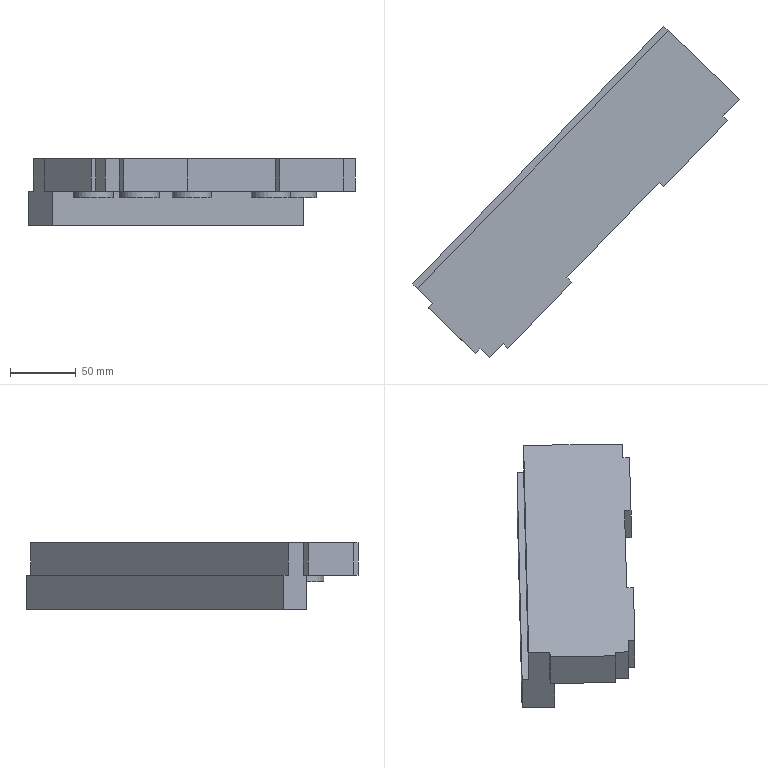Part | NX | features solid 2 | 1 solid | 32 faces | box 248.755 x 252.872 x 51 mm | volume 738406 mm3 | plane 26 | cylinder 5 | spline 1 | commonest cylinder face diameters 30 x5
STEP:
#1=CARTESIAN_POINT('',(577.591,-431.17,45.));
#2=VERTEX_POINT('',#1);
#3=CARTESIAN_POINT('',(577.591,-431.17,20.));
#4=VERTEX_POINT('',#3);
#5=CARTESIAN_POINT('',(577.591,-431.17,45.));
#6=DIRECTION('',(0.,0.,-1.));
#7=VECTOR('',#6,1000.);
#8=LINE('',#5,#7);
#9=EDGE_CURVE('',#2,#4,#8,.T.);
#10=ORIENTED_EDGE('',*,*,#9,.T.);
#11=CARTESIAN_POINT('',(590.046,-418.273,20.));
#12=VERTEX_POINT('',#11);
#13=CARTESIAN_POINT('',(-874.989,-1935.36,20.));
#14=DIRECTION('',(-0.6947,-0.7193,0.));
#15=VECTOR('',#14,1000.);
#16=LINE('',#13,#15);
#17=EDGE_CURVE('',#12,#4,#16,.T.);
#18=ORIENTED_EDGE('',*,*,#17,.F.);
#19=CARTESIAN_POINT('',(590.046,-418.273,45.));
#20=VERTEX_POINT('',#19);
#21=CARTESIAN_POINT('',(590.046,-418.273,70.));
#22=DIRECTION('',(0.,0.,-1.));
#23=VECTOR('',#22,1000.);
#24=LINE('',#21,#23);
#25=EDGE_CURVE('',#20,#12,#24,.T.);
#26=ORIENTED_EDGE('',*,*,#25,.F.);
#27=CARTESIAN_POINT('',(-874.989,-1935.36,45.));
#28=DIRECTION('',(0.6947,0.7193,0.));
#29=VECTOR('',#28,1000.);
#30=LINE('',#27,#29);
#31=EDGE_CURVE('',#2,#20,#30,.T.);
#32=ORIENTED_EDGE('',*,*,#31,.F.);
#33=EDGE_LOOP('',(#10,#18,#26,#32));
#34=FACE_BOUND('',#33,.T.);
#35=CARTESIAN_POINT('',(-874.989,-1935.36,70.));
#36=DIRECTION('',(-0.7193,0.6947,0.));
#37=DIRECTION('',(-0.6947,-0.7193,0.));
#38=AXIS2_PLACEMENT_3D('',#35,#36,#37);
#39=PLANE('',#38);
#40=ADVANCED_FACE('',(#34),#39,.F.);
#41=CARTESIAN_POINT('',(399.709,-615.372,45.));
#42=VERTEX_POINT('',#41);
#43=CARTESIAN_POINT('',(392.516,-608.425,45.));
#44=VERTEX_POINT('',#43);
#45=CARTESIAN_POINT('',(1324.061,-1508.008,45.));
#46=DIRECTION('',(-0.7193,0.6947,0.));
#47=VECTOR('',#46,1000.);
#48=LINE('',#45,#47);
#49=EDGE_CURVE('',#42,#44,#48,.T.);
#50=ORIENTED_EDGE('',*,*,#49,.T.);
#51=CARTESIAN_POINT('',(392.516,-608.425,20.));
#52=VERTEX_POINT('',#51);
#53=CARTESIAN_POINT('',(392.516,-608.425,45.));
#54=DIRECTION('',(0.,0.,1.));
#55=VECTOR('',#54,1000.);
#56=LINE('',#53,#55);
#57=EDGE_CURVE('',#44,#52,#56,.F.);
#58=ORIENTED_EDGE('',*,*,#57,.T.);
#59=CARTESIAN_POINT('',(399.709,-615.372,20.));
#60=VERTEX_POINT('',#59);
#61=CARTESIAN_POINT('',(1324.061,-1508.008,20.));
#62=DIRECTION('',(0.7193,-0.6947,0.));
#63=VECTOR('',#62,1000.);
#64=LINE('',#61,#63);
#65=EDGE_CURVE('',#52,#60,#64,.T.);
#66=ORIENTED_EDGE('',*,*,#65,.T.);
#67=CARTESIAN_POINT('',(399.709,-615.372,70.));
#68=DIRECTION('',(0.,0.,-1.));
#69=VECTOR('',#68,1000.);
#70=LINE('',#67,#69);
#71=EDGE_CURVE('',#42,#60,#70,.T.);
#72=ORIENTED_EDGE('',*,*,#71,.F.);
#73=EDGE_LOOP('',(#50,#58,#66,#72));
#74=FACE_BOUND('',#73,.T.);
#75=CARTESIAN_POINT('',(1324.061,-1508.008,70.));
#76=DIRECTION('',(-0.6947,-0.7193,0.));
#77=DIRECTION('',(0.7193,-0.6947,0.));
#78=AXIS2_PLACEMENT_3D('',#75,#76,#77);
#79=PLANE('',#78);
#80=ADVANCED_FACE('',(#74),#79,.T.);
#81=CARTESIAN_POINT('',(375.617,-574.28,20.));
#82=VERTEX_POINT('',#81);
#83=CARTESIAN_POINT('',(390.617,-574.28,20.));
#84=DIRECTION('',(0.,0.,-1.));
#85=DIRECTION('',(-1.,0.,0.));
#86=AXIS2_PLACEMENT_3D('',#83,#84,#85);
#87=CIRCLE('',#86,15.);
#88=EDGE_CURVE('',#82,#82,#87,.T.);
#89=ORIENTED_EDGE('',*,*,#88,.F.);
#90=EDGE_LOOP('',(#89));
#91=FACE_BOUND('',#90,.T.);
#92=CARTESIAN_POINT('',(510.617,-449.28,20.));
#93=VERTEX_POINT('',#92);
#94=CARTESIAN_POINT('',(525.617,-449.28,20.));
#95=DIRECTION('',(0.,0.,-1.));
#96=DIRECTION('',(-1.,0.,0.));
#97=AXIS2_PLACEMENT_3D('',#94,#95,#96);
#98=CIRCLE('',#97,15.);
#99=EDGE_CURVE('',#93,#93,#98,.T.);
#100=ORIENTED_EDGE('',*,*,#99,.F.);
#101=EDGE_LOOP('',(#100));
#102=FACE_BOUND('',#101,.T.);
#103=CARTESIAN_POINT('',(450.617,-504.28,20.));
#104=VERTEX_POINT('',#103);
#105=CARTESIAN_POINT('',(465.617,-504.28,20.));
#106=DIRECTION('',(0.,0.,-1.));
#107=DIRECTION('',(-1.,0.,0.));
#108=AXIS2_PLACEMENT_3D('',#105,#106,#107);
#109=CIRCLE('',#108,15.);
#110=EDGE_CURVE('',#104,#104,#109,.T.);
#111=ORIENTED_EDGE('',*,*,#110,.F.);
#112=EDGE_LOOP('',(#111));
#113=FACE_BOUND('',#112,.T.);
#114=CARTESIAN_POINT('',(530.617,-419.28,20.));
#115=VERTEX_POINT('',#114);
#116=CARTESIAN_POINT('',(545.617,-419.28,20.));
#117=DIRECTION('',(0.,0.,-1.));
#118=DIRECTION('',(-1.,0.,0.));
#119=AXIS2_PLACEMENT_3D('',#116,#117,#118);
#120=CIRCLE('',#119,15.);
#121=EDGE_CURVE('',#115,#115,#120,.T.);
#122=ORIENTED_EDGE('',*,*,#121,.F.);
#123=EDGE_LOOP('',(#122));
#124=FACE_BOUND('',#123,.T.);
#125=CARTESIAN_POINT('',(410.617,-559.28,20.));
#126=VERTEX_POINT('',#125);
#127=CARTESIAN_POINT('',(425.617,-559.28,20.));
#128=DIRECTION('',(0.,0.,-1.));
#129=DIRECTION('',(-1.,0.,0.));
#130=AXIS2_PLACEMENT_3D('',#127,#128,#129);
#131=CIRCLE('',#130,15.);
#132=EDGE_CURVE('',#126,#126,#131,.T.);
#133=ORIENTED_EDGE('',*,*,#132,.F.);
#134=EDGE_LOOP('',(#133));
#135=FACE_BOUND('',#134,.T.);
#136=ORIENTED_EDGE('',*,*,#65,.F.);
#137=CARTESIAN_POINT('',(389.043,-612.022,20.));
#138=VERTEX_POINT('',#137);
#139=CARTESIAN_POINT('',(392.516,-608.425,20.));
#140=DIRECTION('',(-0.6947,-0.7193,0.));
#141=VECTOR('',#140,1000.);
#142=LINE('',#139,#141);
#143=EDGE_CURVE('',#52,#138,#142,.T.);
#144=ORIENTED_EDGE('',*,*,#143,.T.);
#145=CARTESIAN_POINT('',(353.076,-577.289,20.));
#146=VERTEX_POINT('',#145);
#147=CARTESIAN_POINT('',(432.203,-653.701,20.));
#148=DIRECTION('',(-0.7193,0.6947,0.));
#149=VECTOR('',#148,1000.);
#150=LINE('',#147,#149);
#151=EDGE_CURVE('',#138,#146,#150,.T.);
#152=ORIENTED_EDGE('',*,*,#151,.T.);
#153=CARTESIAN_POINT('',(356.549,-573.692,20.));
#154=VERTEX_POINT('',#153);
#155=CARTESIAN_POINT('',(356.549,-573.692,20.));
#156=DIRECTION('',(-0.6947,-0.7193,0.));
#157=VECTOR('',#156,1000.);
#158=LINE('',#155,#157);
#159=EDGE_CURVE('',#154,#146,#158,.T.);
#160=ORIENTED_EDGE('',*,*,#159,.F.);
#161=CARTESIAN_POINT('',(359.275,-576.324,20.));
#162=VERTEX_POINT('',#161);
#163=CARTESIAN_POINT('',(435.676,-650.105,20.));
#164=DIRECTION('',(-0.7193,0.6947,0.));
#165=VECTOR('',#164,1000.);
#166=LINE('',#163,#165);
#167=EDGE_CURVE('',#162,#154,#166,.T.);
#168=ORIENTED_EDGE('',*,*,#167,.F.);
#169=CARTESIAN_POINT('',(550.275,-379.867,20.));
#170=VERTEX_POINT('',#169);
#171=CARTESIAN_POINT('',(355.898,-579.798,20.));
#172=DIRECTION('',(0.6971,0.717,0.));
#173=VECTOR('',#172,1000.);
#174=LINE('',#171,#173);
#175=EDGE_CURVE('',#162,#170,#174,.T.);
#176=ORIENTED_EDGE('',*,*,#175,.T.);
#177=CARTESIAN_POINT('',(1514.397,-1310.909,20.));
#178=DIRECTION('',(0.7193,-0.6947,0.));
#179=VECTOR('',#178,1000.);
#180=LINE('',#177,#179);
#181=EDGE_CURVE('',#170,#12,#180,.T.);
#182=ORIENTED_EDGE('',*,*,#181,.T.);
#183=ORIENTED_EDGE('',*,*,#17,.T.);
#184=CARTESIAN_POINT('',(581.188,-434.643,20.));
#185=VERTEX_POINT('',#184);
#186=CARTESIAN_POINT('',(577.591,-431.17,20.));
#187=DIRECTION('',(0.7193,-0.6947,0.));
#188=VECTOR('',#187,1000.);
#189=LINE('',#186,#188);
#190=EDGE_CURVE('',#4,#185,#189,.T.);
#191=ORIENTED_EDGE('',*,*,#190,.T.);
#192=CARTESIAN_POINT('',(532.562,-484.997,20.));
#193=VERTEX_POINT('',#192);
#194=CARTESIAN_POINT('',(529.089,-488.593,20.));
#195=DIRECTION('',(0.6947,0.7193,0.));
#196=VECTOR('',#195,1000.);
#197=LINE('',#194,#196);
#198=EDGE_CURVE('',#193,#185,#197,.T.);
#199=ORIENTED_EDGE('',*,*,#198,.F.);
#200=CARTESIAN_POINT('',(528.965,-481.523,20.));
#201=VERTEX_POINT('',#200);
#202=CARTESIAN_POINT('',(528.965,-481.523,20.));
#203=DIRECTION('',(0.7193,-0.6947,0.));
#204=VECTOR('',#203,1000.);
#205=LINE('',#202,#204);
#206=EDGE_CURVE('',#201,#193,#205,.T.);
#207=ORIENTED_EDGE('',*,*,#206,.F.);
#208=CARTESIAN_POINT('',(458.755,-554.228,20.));
#209=VERTEX_POINT('',#208);
#210=CARTESIAN_POINT('',(-874.989,-1935.36,20.));
#211=DIRECTION('',(-0.6947,-0.7193,0.));
#212=VECTOR('',#211,1000.);
#213=LINE('',#210,#212);
#214=EDGE_CURVE('',#201,#209,#213,.T.);
#215=ORIENTED_EDGE('',*,*,#214,.T.);
#216=CARTESIAN_POINT('',(462.352,-557.701,20.));
#217=VERTEX_POINT('',#216);
#218=CARTESIAN_POINT('',(458.755,-554.228,20.));
#219=DIRECTION('',(0.7193,-0.6947,0.));
#220=VECTOR('',#219,1000.);
#221=LINE('',#218,#220);
#222=EDGE_CURVE('',#209,#217,#221,.T.);
#223=ORIENTED_EDGE('',*,*,#222,.T.);
#224=CARTESIAN_POINT('',(413.726,-608.055,20.));
#225=VERTEX_POINT('',#224);
#226=CARTESIAN_POINT('',(396.359,-626.038,20.));
#227=DIRECTION('',(0.6947,0.7193,0.));
#228=VECTOR('',#227,1000.);
#229=LINE('',#226,#228);
#230=EDGE_CURVE('',#225,#217,#229,.T.);
#231=ORIENTED_EDGE('',*,*,#230,.F.);
#232=CARTESIAN_POINT('',(410.129,-604.582,20.));
#233=VERTEX_POINT('',#232);
#234=CARTESIAN_POINT('',(410.129,-604.582,20.));
#235=DIRECTION('',(0.7193,-0.6947,0.));
#236=VECTOR('',#235,1000.);
#237=LINE('',#234,#236);
#238=EDGE_CURVE('',#233,#225,#237,.T.);
#239=ORIENTED_EDGE('',*,*,#238,.F.);
#240=CARTESIAN_POINT('',(-874.989,-1935.36,20.));
#241=DIRECTION('',(-0.6947,-0.7193,0.));
#242=VECTOR('',#241,1000.);
#243=LINE('',#240,#242);
#244=EDGE_CURVE('',#233,#60,#243,.T.);
#245=ORIENTED_EDGE('',*,*,#244,.T.);
#246=EDGE_LOOP('',(#136,#144,#152,#160,#168,#176,#182,#183,#191,#199,#207,#215,#223,#231,#239,#245));
#247=FACE_BOUND('',#246,.T.);
#248=CARTESIAN_POINT('',(389.043,-612.022,20.));
#249=DIRECTION('',(0.,0.,-1.));
#250=DIRECTION('',(-1.,0.,0.));
#251=AXIS2_PLACEMENT_3D('',#248,#249,#250);
#252=PLANE('',#251);
#253=ADVANCED_FACE('',(#91,#102,#113,#124,#135,#247),#252,.T.);
#254=ORIENTED_EDGE('',*,*,#214,.F.);
#255=CARTESIAN_POINT('',(528.965,-481.523,45.));
#256=VERTEX_POINT('',#255);
#257=CARTESIAN_POINT('',(528.965,-481.523,45.));
#258=DIRECTION('',(0.,0.,-1.));
#259=VECTOR('',#258,1000.);
#260=LINE('',#257,#259);
#261=EDGE_CURVE('',#256,#201,#260,.T.);
#262=ORIENTED_EDGE('',*,*,#261,.F.);
#263=CARTESIAN_POINT('',(458.755,-554.228,45.));
#264=VERTEX_POINT('',#263);
#265=CARTESIAN_POINT('',(-874.989,-1935.36,45.));
#266=DIRECTION('',(0.6947,0.7193,0.));
#267=VECTOR('',#266,1000.);
#268=LINE('',#265,#267);
#269=EDGE_CURVE('',#264,#256,#268,.T.);
#270=ORIENTED_EDGE('',*,*,#269,.F.);
#271=CARTESIAN_POINT('',(458.755,-554.228,45.));
#272=DIRECTION('',(0.,0.,-1.));
#273=VECTOR('',#272,1000.);
#274=LINE('',#271,#273);
#275=EDGE_CURVE('',#264,#209,#274,.T.);
#276=ORIENTED_EDGE('',*,*,#275,.T.);
#277=EDGE_LOOP('',(#254,#262,#270,#276));
#278=FACE_BOUND('',#277,.T.);
#279=CARTESIAN_POINT('',(-874.989,-1935.36,70.));
#280=DIRECTION('',(-0.7193,0.6947,0.));
#281=DIRECTION('',(-0.6947,-0.7193,0.));
#282=AXIS2_PLACEMENT_3D('',#279,#280,#281);
#283=PLANE('',#282);
#284=ADVANCED_FACE('',(#278),#283,.F.);
#285=CARTESIAN_POINT('',(410.129,-604.582,45.));
#286=VERTEX_POINT('',#285);
#287=CARTESIAN_POINT('',(-874.989,-1935.36,45.));
#288=DIRECTION('',(0.6947,0.7193,0.));
#289=VECTOR('',#288,1000.);
#290=LINE('',#287,#289);
#291=EDGE_CURVE('',#42,#286,#290,.T.);
#292=ORIENTED_EDGE('',*,*,#291,.T.);
#293=CARTESIAN_POINT('',(413.726,-608.055,45.));
#294=VERTEX_POINT('',#293);
#295=CARTESIAN_POINT('',(410.129,-604.582,45.));
#296=DIRECTION('',(0.7193,-0.6947,0.));
#297=VECTOR('',#296,1000.);
#298=LINE('',#295,#297);
#299=EDGE_CURVE('',#286,#294,#298,.T.);
#300=ORIENTED_EDGE('',*,*,#299,.T.);
#301=CARTESIAN_POINT('',(462.352,-557.701,45.));
#302=VERTEX_POINT('',#301);
#303=CARTESIAN_POINT('',(396.359,-626.038,45.));
#304=DIRECTION('',(0.6947,0.7193,0.));
#305=VECTOR('',#304,1000.);
#306=LINE('',#303,#305);
#307=EDGE_CURVE('',#294,#302,#306,.T.);
#308=ORIENTED_EDGE('',*,*,#307,.T.);
#309=CARTESIAN_POINT('',(458.755,-554.228,45.));
#310=DIRECTION('',(0.7193,-0.6947,0.));
#311=VECTOR('',#310,1000.);
#312=LINE('',#309,#311);
#313=EDGE_CURVE('',#264,#302,#312,.T.);
#314=ORIENTED_EDGE('',*,*,#313,.F.);
#315=ORIENTED_EDGE('',*,*,#269,.T.);
#316=CARTESIAN_POINT('',(532.562,-484.997,45.));
#317=VERTEX_POINT('',#316);
#318=CARTESIAN_POINT('',(528.965,-481.523,45.));
#319=DIRECTION('',(0.7193,-0.6947,0.));
#320=VECTOR('',#319,1000.);
#321=LINE('',#318,#320);
#322=EDGE_CURVE('',#256,#317,#321,.T.);
#323=ORIENTED_EDGE('',*,*,#322,.T.);
#324=CARTESIAN_POINT('',(581.188,-434.643,45.));
#325=VERTEX_POINT('',#324);
#326=CARTESIAN_POINT('',(529.089,-488.593,45.));
#327=DIRECTION('',(0.6947,0.7193,0.));
#328=VECTOR('',#327,1000.);
#329=LINE('',#326,#328);
#330=EDGE_CURVE('',#317,#325,#329,.T.);
#331=ORIENTED_EDGE('',*,*,#330,.T.);
#332=CARTESIAN_POINT('',(577.591,-431.17,45.));
#333=DIRECTION('',(0.7193,-0.6947,0.));
#334=VECTOR('',#333,1000.);
#335=LINE('',#332,#334);
#336=EDGE_CURVE('',#2,#325,#335,.T.);
#337=ORIENTED_EDGE('',*,*,#336,.F.);
#338=ORIENTED_EDGE('',*,*,#31,.T.);
#339=CARTESIAN_POINT('',(535.888,-365.973,45.));
#340=VERTEX_POINT('',#339);
#341=CARTESIAN_POINT('',(1514.397,-1310.909,45.));
#342=DIRECTION('',(-0.7193,0.6947,0.));
#343=VECTOR('',#342,1000.);
#344=LINE('',#341,#343);
#345=EDGE_CURVE('',#20,#340,#344,.T.);
#346=ORIENTED_EDGE('',*,*,#345,.T.);
#347=CARTESIAN_POINT('',(344.888,-562.431,45.));
#348=VERTEX_POINT('',#347);
#349=CARTESIAN_POINT('',(536.574,-365.269,45.));
#350=DIRECTION('',(-0.6971,-0.717,0.));
#351=VECTOR('',#350,1000.);
#352=LINE('',#349,#351);
#353=EDGE_CURVE('',#340,#348,#352,.T.);
#354=ORIENTED_EDGE('',*,*,#353,.T.);
#355=CARTESIAN_POINT('',(356.549,-573.692,45.));
#356=VERTEX_POINT('',#355);
#357=CARTESIAN_POINT('',(1324.061,-1508.008,45.));
#358=DIRECTION('',(-0.7193,0.6947,0.));
#359=VECTOR('',#358,1000.);
#360=LINE('',#357,#359);
#361=EDGE_CURVE('',#356,#348,#360,.T.);
#362=ORIENTED_EDGE('',*,*,#361,.F.);
#363=CARTESIAN_POINT('',(353.076,-577.289,45.));
#364=VERTEX_POINT('',#363);
#365=CARTESIAN_POINT('',(356.549,-573.692,45.));
#366=DIRECTION('',(-0.6947,-0.7193,0.));
#367=VECTOR('',#366,1000.);
#368=LINE('',#365,#367);
#369=EDGE_CURVE('',#356,#364,#368,.T.);
#370=ORIENTED_EDGE('',*,*,#369,.T.);
#371=CARTESIAN_POINT('',(389.043,-612.022,45.));
#372=VERTEX_POINT('',#371);
#373=CARTESIAN_POINT('',(432.203,-653.701,45.));
#374=DIRECTION('',(-0.7193,0.6947,0.));
#375=VECTOR('',#374,1000.);
#376=LINE('',#373,#375);
#377=EDGE_CURVE('',#372,#364,#376,.T.);
#378=ORIENTED_EDGE('',*,*,#377,.F.);
#379=CARTESIAN_POINT('',(392.516,-608.425,45.));
#380=DIRECTION('',(-0.6947,-0.7193,0.));
#381=VECTOR('',#380,1000.);
#382=LINE('',#379,#381);
#383=EDGE_CURVE('',#44,#372,#382,.T.);
#384=ORIENTED_EDGE('',*,*,#383,.F.);
#385=ORIENTED_EDGE('',*,*,#49,.F.);
#386=EDGE_LOOP('',(#292,#300,#308,#314,#315,#323,#331,#337,#338,#346,#354,#362,#370,#378,#384,#385));
#387=FACE_BOUND('',#386,.T.);
#388=CARTESIAN_POINT('',(631.984,-1285.265,45.));
#389=DIRECTION('',(0.,0.,1.));
#390=DIRECTION('',(1.,0.,0.));
#391=AXIS2_PLACEMENT_3D('',#388,#389,#390);
#392=PLANE('',#391);
#393=ADVANCED_FACE('',(#387),#392,.T.);
#394=CARTESIAN_POINT('',(344.888,-562.431,20.));
#395=VERTEX_POINT('',#394);
#396=CARTESIAN_POINT('',(344.888,-562.431,70.));
#397=DIRECTION('',(0.,0.,1.));
#398=VECTOR('',#397,1000.);
#399=LINE('',#396,#398);
#400=EDGE_CURVE('',#395,#348,#399,.T.);
#401=ORIENTED_EDGE('',*,*,#400,.T.);
#402=ORIENTED_EDGE('',*,*,#353,.F.);
#403=CARTESIAN_POINT('',(535.888,-365.973,20.));
#404=VERTEX_POINT('',#403);
#405=CARTESIAN_POINT('',(535.888,-365.973,70.));
#406=DIRECTION('',(0.,0.,1.));
#407=VECTOR('',#406,1000.);
#408=LINE('',#405,#407);
#409=EDGE_CURVE('',#340,#404,#408,.F.);
#410=ORIENTED_EDGE('',*,*,#409,.T.);
#411=CARTESIAN_POINT('',(536.574,-365.269,20.));
#412=DIRECTION('',(0.6971,0.717,0.));
#413=VECTOR('',#412,1000.);
#414=LINE('',#411,#413);
#415=EDGE_CURVE('',#395,#404,#414,.T.);
#416=ORIENTED_EDGE('',*,*,#415,.F.);
#417=EDGE_LOOP('',(#401,#402,#410,#416));
#418=FACE_BOUND('',#417,.T.);
#419=CARTESIAN_POINT('',(536.574,-365.269,70.));
#420=DIRECTION('',(0.717,-0.6971,0.));
#421=DIRECTION('',(0.6971,0.717,0.));
#422=AXIS2_PLACEMENT_3D('',#419,#420,#421);
#423=PLANE('',#422);
#424=ADVANCED_FACE('',(#418),#423,.F.);
#425=ORIENTED_EDGE('',*,*,#181,.F.);
#426=CARTESIAN_POINT('',(550.275,-379.867,-6.));
#427=VERTEX_POINT('',#426);
#428=CARTESIAN_POINT('',(550.275,-379.867,-10.));
#429=DIRECTION('',(0.,0.,1.));
#430=VECTOR('',#429,1000.);
#431=LINE('',#428,#430);
#432=EDGE_CURVE('',#427,#170,#431,.T.);
#433=ORIENTED_EDGE('',*,*,#432,.F.);
#434=CARTESIAN_POINT('',(532.292,-362.5,-6.));
#435=VERTEX_POINT('',#434);
#436=CARTESIAN_POINT('',(1514.397,-1310.909,-6.));
#437=DIRECTION('',(-0.7193,0.6947,0.));
#438=VECTOR('',#437,1000.);
#439=LINE('',#436,#438);
#440=EDGE_CURVE('',#427,#435,#439,.T.);
#441=ORIENTED_EDGE('',*,*,#440,.T.);
#442=CARTESIAN_POINT('',(532.292,-362.5,20.));
#443=VERTEX_POINT('',#442);
#444=CARTESIAN_POINT('',(532.292,-362.5,70.));
#445=DIRECTION('',(0.,0.,-1.));
#446=VECTOR('',#445,1000.);
#447=LINE('',#444,#446);
#448=EDGE_CURVE('',#443,#435,#447,.T.);
#449=ORIENTED_EDGE('',*,*,#448,.F.);
#450=CARTESIAN_POINT('',(532.292,-362.5,20.));
#451=CARTESIAN_POINT('',(533.49,-363.658,20.));
#452=CARTESIAN_POINT('',(534.689,-364.816,20.));
#453=CARTESIAN_POINT('',(535.888,-365.973,20.));
#454=B_SPLINE_CURVE_WITH_KNOTS('',3,(#450,#451,#452,#453),.UNSPECIFIED.,.F.,.F.,(4,4),(0.03993,0.04493),.UNSPECIFIED.);
#455=EDGE_CURVE('',#443,#404,#454,.T.);
#456=ORIENTED_EDGE('',*,*,#455,.T.);
#457=ORIENTED_EDGE('',*,*,#409,.F.);
#458=ORIENTED_EDGE('',*,*,#345,.F.);
#459=ORIENTED_EDGE('',*,*,#25,.T.);
#460=EDGE_LOOP('',(#425,#433,#441,#449,#456,#457,#458,#459));
#461=FACE_BOUND('',#460,.T.);
#462=CARTESIAN_POINT('',(1514.397,-1310.909,70.));
#463=DIRECTION('',(-0.6947,-0.7193,0.));
#464=DIRECTION('',(0.7193,-0.6947,0.));
#465=AXIS2_PLACEMENT_3D('',#462,#463,#464);
#466=PLANE('',#465);
#467=ADVANCED_FACE('',(#461),#466,.F.);
#468=ORIENTED_EDGE('',*,*,#244,.F.);
#469=CARTESIAN_POINT('',(410.129,-604.582,45.));
#470=DIRECTION('',(0.,0.,1.));
#471=VECTOR('',#470,1000.);
#472=LINE('',#469,#471);
#473=EDGE_CURVE('',#286,#233,#472,.F.);
#474=ORIENTED_EDGE('',*,*,#473,.F.);
#475=ORIENTED_EDGE('',*,*,#291,.F.);
#476=ORIENTED_EDGE('',*,*,#71,.T.);
#477=EDGE_LOOP('',(#468,#474,#475,#476));
#478=FACE_BOUND('',#477,.T.);
#479=CARTESIAN_POINT('',(-874.989,-1935.36,70.));
#480=DIRECTION('',(-0.7193,0.6947,0.));
#481=DIRECTION('',(-0.6947,-0.7193,0.));
#482=AXIS2_PLACEMENT_3D('',#479,#480,#481);
#483=PLANE('',#482);
#484=ADVANCED_FACE('',(#478),#483,.F.);
#485=CARTESIAN_POINT('',(356.549,-573.692,45.));
#486=DIRECTION('',(0.,0.,-1.));
#487=VECTOR('',#486,1000.);
#488=LINE('',#485,#487);
#489=EDGE_CURVE('',#356,#154,#488,.T.);
#490=ORIENTED_EDGE('',*,*,#489,.F.);
#491=ORIENTED_EDGE('',*,*,#361,.T.);
#492=ORIENTED_EDGE('',*,*,#400,.F.);
#493=CARTESIAN_POINT('',(341.291,-558.958,20.));
#494=VERTEX_POINT('',#493);
#495=CARTESIAN_POINT('',(341.291,-558.958,20.));
#496=CARTESIAN_POINT('',(342.49,-560.116,20.));
#497=CARTESIAN_POINT('',(343.689,-561.273,20.));
#498=CARTESIAN_POINT('',(344.888,-562.431,20.));
#499=B_SPLINE_CURVE_WITH_KNOTS('',3,(#495,#496,#497,#498),.UNSPECIFIED.,.F.,.F.,(4,4),(0.01164,0.01664),.UNSPECIFIED.);
#500=EDGE_CURVE('',#494,#395,#499,.T.);
#501=ORIENTED_EDGE('',*,*,#500,.F.);
#502=CARTESIAN_POINT('',(341.291,-558.958,-6.));
#503=VERTEX_POINT('',#502);
#504=CARTESIAN_POINT('',(341.291,-558.958,70.));
#505=DIRECTION('',(0.,0.,-1.));
#506=VECTOR('',#505,1000.);
#507=LINE('',#504,#506);
#508=EDGE_CURVE('',#494,#503,#507,.T.);
#509=ORIENTED_EDGE('',*,*,#508,.T.);
#510=CARTESIAN_POINT('',(359.275,-576.324,-6.));
#511=VERTEX_POINT('',#510);
#512=CARTESIAN_POINT('',(1324.061,-1508.008,-6.));
#513=DIRECTION('',(-0.7193,0.6947,0.));
#514=VECTOR('',#513,1000.);
#515=LINE('',#512,#514);
#516=EDGE_CURVE('',#511,#503,#515,.T.);
#517=ORIENTED_EDGE('',*,*,#516,.F.);
#518=CARTESIAN_POINT('',(359.275,-576.324,70.));
#519=DIRECTION('',(0.,0.,-1.));
#520=VECTOR('',#519,1000.);
#521=LINE('',#518,#520);
#522=EDGE_CURVE('',#162,#511,#521,.T.);
#523=ORIENTED_EDGE('',*,*,#522,.F.);
#524=ORIENTED_EDGE('',*,*,#167,.T.);
#525=EDGE_LOOP('',(#490,#491,#492,#501,#509,#517,#523,#524));
#526=FACE_BOUND('',#525,.T.);
#527=CARTESIAN_POINT('',(1324.061,-1508.008,70.));
#528=DIRECTION('',(-0.6947,-0.7193,0.));
#529=DIRECTION('',(0.7193,-0.6947,0.));
#530=AXIS2_PLACEMENT_3D('',#527,#528,#529);
#531=PLANE('',#530);
#532=ADVANCED_FACE('',(#526),#531,.T.);
#533=CARTESIAN_POINT('',(462.352,-557.701,45.));
#534=DIRECTION('',(0.,0.,-1.));
#535=VECTOR('',#534,1000.);
#536=LINE('',#533,#535);
#537=EDGE_CURVE('',#302,#217,#536,.T.);
#538=ORIENTED_EDGE('',*,*,#537,.T.);
#539=ORIENTED_EDGE('',*,*,#222,.F.);
#540=ORIENTED_EDGE('',*,*,#275,.F.);
#541=ORIENTED_EDGE('',*,*,#313,.T.);
#542=EDGE_LOOP('',(#538,#539,#540,#541));
#543=FACE_BOUND('',#542,.T.);
#544=CARTESIAN_POINT('',(458.755,-554.228,45.));
#545=DIRECTION('',(-0.6947,-0.7193,0.));
#546=DIRECTION('',(0.7193,-0.6947,0.));
#547=AXIS2_PLACEMENT_3D('',#544,#545,#546);
#548=PLANE('',#547);
#549=ADVANCED_FACE('',(#543),#548,.F.);
#550=CARTESIAN_POINT('',(413.726,-608.055,45.));
#551=DIRECTION('',(0.,0.,1.));
#552=VECTOR('',#551,1000.);
#553=LINE('',#550,#552);
#554=EDGE_CURVE('',#294,#225,#553,.F.);
#555=ORIENTED_EDGE('',*,*,#554,.F.);
#556=ORIENTED_EDGE('',*,*,#299,.F.);
#557=ORIENTED_EDGE('',*,*,#473,.T.);
#558=ORIENTED_EDGE('',*,*,#238,.T.);
#559=EDGE_LOOP('',(#555,#556,#557,#558));
#560=FACE_BOUND('',#559,.T.);
#561=CARTESIAN_POINT('',(410.129,-604.582,45.));
#562=DIRECTION('',(-0.6947,-0.7193,0.));
#563=DIRECTION('',(0.7193,-0.6947,0.));
#564=AXIS2_PLACEMENT_3D('',#561,#562,#563);
#565=PLANE('',#564);
#566=ADVANCED_FACE('',(#560),#565,.T.);
#567=ORIENTED_EDGE('',*,*,#537,.F.);
#568=ORIENTED_EDGE('',*,*,#307,.F.);
#569=ORIENTED_EDGE('',*,*,#554,.T.);
#570=ORIENTED_EDGE('',*,*,#230,.T.);
#571=EDGE_LOOP('',(#567,#568,#569,#570));
#572=FACE_BOUND('',#571,.T.);
#573=CARTESIAN_POINT('',(396.359,-626.038,45.));
#574=DIRECTION('',(0.7193,-0.6947,0.));
#575=DIRECTION('',(0.,0.,-1.));
#576=AXIS2_PLACEMENT_3D('',#573,#574,#575);
#577=PLANE('',#576);
#578=ADVANCED_FACE('',(#572),#577,.T.);
#579=ORIENTED_EDGE('',*,*,#440,.F.);
#580=CARTESIAN_POINT('',(137.46,-804.477,-6.));
#581=DIRECTION('',(-0.6971,-0.717,0.));
#582=VECTOR('',#581,1000.);
#583=LINE('',#580,#582);
#584=EDGE_CURVE('',#427,#511,#583,.T.);
#585=ORIENTED_EDGE('',*,*,#584,.T.);
#586=ORIENTED_EDGE('',*,*,#516,.T.);
#587=CARTESIAN_POINT('',(532.989,-361.783,-6.));
#588=DIRECTION('',(-0.6971,-0.717,0.));
#589=VECTOR('',#588,1000.);
#590=LINE('',#587,#589);
#591=EDGE_CURVE('',#435,#503,#590,.T.);
#592=ORIENTED_EDGE('',*,*,#591,.F.);
#593=EDGE_LOOP('',(#579,#585,#586,#592));
#594=FACE_BOUND('',#593,.T.);
#595=CARTESIAN_POINT('',(631.984,-1285.265,-6.));
#596=DIRECTION('',(0.,0.,1.));
#597=DIRECTION('',(1.,0.,0.));
#598=AXIS2_PLACEMENT_3D('',#595,#596,#597);
#599=PLANE('',#598);
#600=ADVANCED_FACE('',(#594),#599,.F.);
#601=ORIENTED_EDGE('',*,*,#508,.F.);
#602=CARTESIAN_POINT('',(532.292,-362.5,20.));
#603=CARTESIAN_POINT('',(468.625,-427.986,20.));
#604=CARTESIAN_POINT('',(404.958,-493.472,20.));
#605=CARTESIAN_POINT('',(341.291,-558.958,20.));
#606=B_SPLINE_CURVE_WITH_KNOTS('',3,(#602,#603,#604,#605),.UNSPECIFIED.,.F.,.F.,(4,4),(1.169,1.443),.UNSPECIFIED.);
#607=EDGE_CURVE('',#443,#494,#606,.T.);
#608=ORIENTED_EDGE('',*,*,#607,.F.);
#609=ORIENTED_EDGE('',*,*,#448,.T.);
#610=ORIENTED_EDGE('',*,*,#591,.T.);
#611=EDGE_LOOP('',(#601,#608,#609,#610));
#612=FACE_BOUND('',#611,.T.);
#613=CARTESIAN_POINT('',(532.989,-361.783,70.));
#614=DIRECTION('',(0.717,-0.6971,0.));
#615=DIRECTION('',(0.6971,0.717,0.));
#616=AXIS2_PLACEMENT_3D('',#613,#614,#615);
#617=PLANE('',#616);
#618=ADVANCED_FACE('',(#612),#617,.F.);
#619=ORIENTED_EDGE('',*,*,#500,.T.);
#620=ORIENTED_EDGE('',*,*,#415,.T.);
#621=ORIENTED_EDGE('',*,*,#455,.F.);
#622=ORIENTED_EDGE('',*,*,#607,.T.);
#623=EDGE_LOOP('',(#619,#620,#621,#622));
#624=FACE_BOUND('',#623,.T.);
#625=CARTESIAN_POINT('',(532.989,-361.783,20.));
#626=CARTESIAN_POINT('',(536.574,-365.269,20.));
#627=CARTESIAN_POINT('',(465.155,-431.554,20.));
#628=CARTESIAN_POINT('',(468.74,-435.04,20.));
#629=CARTESIAN_POINT('',(409.209,-489.1,20.));
#630=CARTESIAN_POINT('',(412.794,-492.585,20.));
#631=CARTESIAN_POINT('',(341.291,-558.958,20.));
#632=CARTESIAN_POINT('',(344.876,-562.443,20.));
#633=B_SPLINE_SURFACE_WITH_KNOTS('',3,1,((#625,#626),(#627,#628),(#629,#630),(#631,#632)),.SURF_OF_LINEAR_EXTRUSION.,.F.,.F.,.F.,(4,4),(2,2),(0.,1.),(0.,1.),.PIECEWISE_BEZIER_KNOTS.);
#634=ADVANCED_FACE('',(#624),#633,.T.);
#635=ORIENTED_EDGE('',*,*,#175,.F.);
#636=ORIENTED_EDGE('',*,*,#522,.T.);
#637=ORIENTED_EDGE('',*,*,#584,.F.);
#638=ORIENTED_EDGE('',*,*,#432,.T.);
#639=EDGE_LOOP('',(#635,#636,#637,#638));
#640=FACE_BOUND('',#639,.T.);
#641=CARTESIAN_POINT('',(550.216,-379.927,-10.));
#642=DIRECTION('',(-0.717,0.6971,0.));
#643=DIRECTION('',(-0.6971,-0.717,0.));
#644=AXIS2_PLACEMENT_3D('',#641,#642,#643);
#645=PLANE('',#644);
#646=ADVANCED_FACE('',(#640),#645,.F.);
#647=CARTESIAN_POINT('',(353.076,-577.289,45.));
#648=DIRECTION('',(0.,0.,-1.));
#649=VECTOR('',#648,1000.);
#650=LINE('',#647,#649);
#651=EDGE_CURVE('',#364,#146,#650,.T.);
#652=ORIENTED_EDGE('',*,*,#651,.F.);
#653=ORIENTED_EDGE('',*,*,#369,.F.);
#654=ORIENTED_EDGE('',*,*,#489,.T.);
#655=ORIENTED_EDGE('',*,*,#159,.T.);
#656=EDGE_LOOP('',(#652,#653,#654,#655));
#657=FACE_BOUND('',#656,.T.);
#658=CARTESIAN_POINT('',(356.549,-573.692,45.));
#659=DIRECTION('',(-0.7193,0.6947,0.));
#660=DIRECTION('',(-0.6947,-0.7193,0.));
#661=AXIS2_PLACEMENT_3D('',#658,#659,#660);
#662=PLANE('',#661);
#663=ADVANCED_FACE('',(#657),#662,.T.);
#664=CARTESIAN_POINT('',(389.043,-612.022,45.));
#665=DIRECTION('',(0.,0.,1.));
#666=VECTOR('',#665,1000.);
#667=LINE('',#664,#666);
#668=EDGE_CURVE('',#372,#138,#667,.F.);
#669=ORIENTED_EDGE('',*,*,#668,.T.);
#670=ORIENTED_EDGE('',*,*,#143,.F.);
#671=ORIENTED_EDGE('',*,*,#57,.F.);
#672=ORIENTED_EDGE('',*,*,#383,.T.);
#673=EDGE_LOOP('',(#669,#670,#671,#672));
#674=FACE_BOUND('',#673,.T.);
#675=CARTESIAN_POINT('',(392.516,-608.425,45.));
#676=DIRECTION('',(-0.7193,0.6947,0.));
#677=DIRECTION('',(-0.6947,-0.7193,0.));
#678=AXIS2_PLACEMENT_3D('',#675,#676,#677);
#679=PLANE('',#678);
#680=ADVANCED_FACE('',(#674),#679,.F.);
#681=ORIENTED_EDGE('',*,*,#651,.T.);
#682=ORIENTED_EDGE('',*,*,#151,.F.);
#683=ORIENTED_EDGE('',*,*,#668,.F.);
#684=ORIENTED_EDGE('',*,*,#377,.T.);
#685=EDGE_LOOP('',(#681,#682,#683,#684));
#686=FACE_BOUND('',#685,.T.);
#687=CARTESIAN_POINT('',(432.203,-653.701,45.));
#688=DIRECTION('',(0.6947,0.7193,0.));
#689=DIRECTION('',(0.,0.,-1.));
#690=AXIS2_PLACEMENT_3D('',#687,#688,#689);
#691=PLANE('',#690);
#692=ADVANCED_FACE('',(#686),#691,.F.);
#693=CARTESIAN_POINT('',(581.188,-434.643,45.));
#694=DIRECTION('',(0.,0.,-1.));
#695=VECTOR('',#694,1000.);
#696=LINE('',#693,#695);
#697=EDGE_CURVE('',#325,#185,#696,.T.);
#698=ORIENTED_EDGE('',*,*,#697,.T.);
#699=ORIENTED_EDGE('',*,*,#190,.F.);
#700=ORIENTED_EDGE('',*,*,#9,.F.);
#701=ORIENTED_EDGE('',*,*,#336,.T.);
#702=EDGE_LOOP('',(#698,#699,#700,#701));
#703=FACE_BOUND('',#702,.T.);
#704=CARTESIAN_POINT('',(577.591,-431.17,45.));
#705=DIRECTION('',(-0.6947,-0.7193,0.));
#706=DIRECTION('',(0.7193,-0.6947,0.));
#707=AXIS2_PLACEMENT_3D('',#704,#705,#706);
#708=PLANE('',#707);
#709=ADVANCED_FACE('',(#703),#708,.F.);
#710=CARTESIAN_POINT('',(532.562,-484.997,45.));
#711=DIRECTION('',(0.,0.,-1.));
#712=VECTOR('',#711,1000.);
#713=LINE('',#710,#712);
#714=EDGE_CURVE('',#317,#193,#713,.T.);
#715=ORIENTED_EDGE('',*,*,#714,.F.);
#716=ORIENTED_EDGE('',*,*,#322,.F.);
#717=ORIENTED_EDGE('',*,*,#261,.T.);
#718=ORIENTED_EDGE('',*,*,#206,.T.);
#719=EDGE_LOOP('',(#715,#716,#717,#718));
#720=FACE_BOUND('',#719,.T.);
#721=CARTESIAN_POINT('',(528.965,-481.523,45.));
#722=DIRECTION('',(-0.6947,-0.7193,0.));
#723=DIRECTION('',(0.7193,-0.6947,0.));
#724=AXIS2_PLACEMENT_3D('',#721,#722,#723);
#725=PLANE('',#724);
#726=ADVANCED_FACE('',(#720),#725,.T.);
#727=ORIENTED_EDGE('',*,*,#697,.F.);
#728=ORIENTED_EDGE('',*,*,#330,.F.);
#729=ORIENTED_EDGE('',*,*,#714,.T.);
#730=ORIENTED_EDGE('',*,*,#198,.T.);
#731=EDGE_LOOP('',(#727,#728,#729,#730));
#732=FACE_BOUND('',#731,.T.);
#733=CARTESIAN_POINT('',(529.089,-488.593,45.));
#734=DIRECTION('',(0.7193,-0.6947,0.));
#735=DIRECTION('',(0.,0.,-1.));
#736=AXIS2_PLACEMENT_3D('',#733,#734,#735);
#737=PLANE('',#736);
#738=ADVANCED_FACE('',(#732),#737,.T.);
#739=CARTESIAN_POINT('',(440.617,-559.28,15.));
#740=VERTEX_POINT('',#739);
#741=CARTESIAN_POINT('',(425.617,-559.28,15.));
#742=DIRECTION('',(0.,0.,1.));
#743=DIRECTION('',(1.,0.,0.));
#744=AXIS2_PLACEMENT_3D('',#741,#742,#743);
#745=CIRCLE('',#744,15.);
#746=EDGE_CURVE('',#740,#740,#745,.T.);
#747=ORIENTED_EDGE('',*,*,#746,.T.);
#748=EDGE_LOOP('',(#747));
#749=FACE_BOUND('',#748,.T.);
#750=ORIENTED_EDGE('',*,*,#132,.T.);
#751=EDGE_LOOP('',(#750));
#752=FACE_BOUND('',#751,.T.);
#753=CARTESIAN_POINT('',(425.617,-559.28,15.));
#754=DIRECTION('',(0.,0.,1.));
#755=DIRECTION('',(1.,0.,0.));
#756=AXIS2_PLACEMENT_3D('',#753,#754,#755);
#757=CYLINDRICAL_SURFACE('',#756,15.);
#758=ADVANCED_FACE('',(#749,#752),#757,.T.);
#759=ORIENTED_EDGE('',*,*,#746,.F.);
#760=EDGE_LOOP('',(#759));
#761=FACE_BOUND('',#760,.T.);
#762=CARTESIAN_POINT('',(425.617,-559.28,15.));
#763=DIRECTION('',(0.,0.,1.));
#764=DIRECTION('',(1.,0.,0.));
#765=AXIS2_PLACEMENT_3D('',#762,#763,#764);
#766=PLANE('',#765);
#767=ADVANCED_FACE('',(#761),#766,.F.);
#768=CARTESIAN_POINT('',(560.617,-419.28,15.));
#769=VERTEX_POINT('',#768);
#770=CARTESIAN_POINT('',(545.617,-419.28,15.));
#771=DIRECTION('',(0.,0.,1.));
#772=DIRECTION('',(1.,0.,0.));
#773=AXIS2_PLACEMENT_3D('',#770,#771,#772);
#774=CIRCLE('',#773,15.);
#775=EDGE_CURVE('',#769,#769,#774,.T.);
#776=ORIENTED_EDGE('',*,*,#775,.T.);
#777=EDGE_LOOP('',(#776));
#778=FACE_BOUND('',#777,.T.);
#779=ORIENTED_EDGE('',*,*,#121,.T.);
#780=EDGE_LOOP('',(#779));
#781=FACE_BOUND('',#780,.T.);
#782=CARTESIAN_POINT('',(545.617,-419.28,15.));
#783=DIRECTION('',(0.,0.,1.));
#784=DIRECTION('',(1.,0.,0.));
#785=AXIS2_PLACEMENT_3D('',#782,#783,#784);
#786=CYLINDRICAL_SURFACE('',#785,15.);
#787=ADVANCED_FACE('',(#778,#781),#786,.T.);
#788=ORIENTED_EDGE('',*,*,#775,.F.);
#789=EDGE_LOOP('',(#788));
#790=FACE_BOUND('',#789,.T.);
#791=CARTESIAN_POINT('',(545.617,-419.28,15.));
#792=DIRECTION('',(0.,0.,1.));
#793=DIRECTION('',(1.,0.,0.));
#794=AXIS2_PLACEMENT_3D('',#791,#792,#793);
#795=PLANE('',#794);
#796=ADVANCED_FACE('',(#790),#795,.F.);
#797=CARTESIAN_POINT('',(480.617,-504.28,15.));
#798=VERTEX_POINT('',#797);
#799=CARTESIAN_POINT('',(465.617,-504.28,15.));
#800=DIRECTION('',(0.,0.,1.));
#801=DIRECTION('',(1.,0.,0.));
#802=AXIS2_PLACEMENT_3D('',#799,#800,#801);
#803=CIRCLE('',#802,15.);
#804=EDGE_CURVE('',#798,#798,#803,.T.);
#805=ORIENTED_EDGE('',*,*,#804,.T.);
#806=EDGE_LOOP('',(#805));
#807=FACE_BOUND('',#806,.T.);
#808=ORIENTED_EDGE('',*,*,#110,.T.);
#809=EDGE_LOOP('',(#808));
#810=FACE_BOUND('',#809,.T.);
#811=CARTESIAN_POINT('',(465.617,-504.28,15.));
#812=DIRECTION('',(0.,0.,1.));
#813=DIRECTION('',(1.,0.,0.));
#814=AXIS2_PLACEMENT_3D('',#811,#812,#813);
#815=CYLINDRICAL_SURFACE('',#814,15.);
#816=ADVANCED_FACE('',(#807,#810),#815,.T.);
#817=ORIENTED_EDGE('',*,*,#804,.F.);
#818=EDGE_LOOP('',(#817));
#819=FACE_BOUND('',#818,.T.);
#820=CARTESIAN_POINT('',(465.617,-504.28,15.));
#821=DIRECTION('',(0.,0.,1.));
#822=DIRECTION('',(1.,0.,0.));
#823=AXIS2_PLACEMENT_3D('',#820,#821,#822);
#824=PLANE('',#823);
#825=ADVANCED_FACE('',(#819),#824,.F.);
#826=CARTESIAN_POINT('',(540.617,-449.28,15.));
#827=VERTEX_POINT('',#826);
#828=CARTESIAN_POINT('',(525.617,-449.28,15.));
#829=DIRECTION('',(0.,0.,1.));
#830=DIRECTION('',(1.,0.,0.));
#831=AXIS2_PLACEMENT_3D('',#828,#829,#830);
#832=CIRCLE('',#831,15.);
#833=EDGE_CURVE('',#827,#827,#832,.T.);
#834=ORIENTED_EDGE('',*,*,#833,.T.);
#835=EDGE_LOOP('',(#834));
#836=FACE_BOUND('',#835,.T.);
#837=ORIENTED_EDGE('',*,*,#99,.T.);
#838=EDGE_LOOP('',(#837));
#839=FACE_BOUND('',#838,.T.);
#840=CARTESIAN_POINT('',(525.617,-449.28,15.));
#841=DIRECTION('',(0.,0.,1.));
#842=DIRECTION('',(1.,0.,0.));
#843=AXIS2_PLACEMENT_3D('',#840,#841,#842);
#844=CYLINDRICAL_SURFACE('',#843,15.);
#845=ADVANCED_FACE('',(#836,#839),#844,.T.);
#846=ORIENTED_EDGE('',*,*,#833,.F.);
#847=EDGE_LOOP('',(#846));
#848=FACE_BOUND('',#847,.T.);
#849=CARTESIAN_POINT('',(525.617,-449.28,15.));
#850=DIRECTION('',(0.,0.,1.));
#851=DIRECTION('',(1.,0.,0.));
#852=AXIS2_PLACEMENT_3D('',#849,#850,#851);
#853=PLANE('',#852);
#854=ADVANCED_FACE('',(#848),#853,.F.);
#855=CARTESIAN_POINT('',(405.617,-574.28,15.));
#856=VERTEX_POINT('',#855);
#857=CARTESIAN_POINT('',(390.617,-574.28,15.));
#858=DIRECTION('',(0.,0.,1.));
#859=DIRECTION('',(1.,0.,0.));
#860=AXIS2_PLACEMENT_3D('',#857,#858,#859);
#861=CIRCLE('',#860,15.);
#862=EDGE_CURVE('',#856,#856,#861,.T.);
#863=ORIENTED_EDGE('',*,*,#862,.T.);
#864=EDGE_LOOP('',(#863));
#865=FACE_BOUND('',#864,.T.);
#866=ORIENTED_EDGE('',*,*,#88,.T.);
#867=EDGE_LOOP('',(#866));
#868=FACE_BOUND('',#867,.T.);
#869=CARTESIAN_POINT('',(390.617,-574.28,15.));
#870=DIRECTION('',(0.,0.,1.));
#871=DIRECTION('',(1.,0.,0.));
#872=AXIS2_PLACEMENT_3D('',#869,#870,#871);
#873=CYLINDRICAL_SURFACE('',#872,15.);
#874=ADVANCED_FACE('',(#865,#868),#873,.T.);
#875=ORIENTED_EDGE('',*,*,#862,.F.);
#876=EDGE_LOOP('',(#875));
#877=FACE_BOUND('',#876,.T.);
#878=CARTESIAN_POINT('',(390.617,-574.28,15.));
#879=DIRECTION('',(0.,0.,1.));
#880=DIRECTION('',(1.,0.,0.));
#881=AXIS2_PLACEMENT_3D('',#878,#879,#880);
#882=PLANE('',#881);
#883=ADVANCED_FACE('',(#877),#882,.F.);
#884=CLOSED_SHELL('',(#40,#80,#253,#284,#393,#424,#467,#484,#532,#549,#566,#578,#600,#618,#634,#646,#663,#680,#692,#709,#726,#738,#758,#767,#787,#796,#816,#825,#845,#854,#874,#883));
#885=MANIFOLD_SOLID_BREP('',#884);
#886=(LENGTH_UNIT()NAMED_UNIT(*)SI_UNIT(.MILLI.,.METRE.));
#887=UNCERTAINTY_MEASURE_WITH_UNIT(LENGTH_MEASURE(0.0508),#886,'','');
#888=(NAMED_UNIT(*)PLANE_ANGLE_UNIT()SI_UNIT($,.RADIAN.));
#889=(NAMED_UNIT(*)SI_UNIT($,.STERADIAN.)SOLID_ANGLE_UNIT());
#890=(GEOMETRIC_REPRESENTATION_CONTEXT(3)GLOBAL_UNCERTAINTY_ASSIGNED_CONTEXT((#887))GLOBAL_UNIT_ASSIGNED_CONTEXT((#886,#888,#889))REPRESENTATION_CONTEXT('',''));
#891=ADVANCED_BREP_SHAPE_REPRESENTATION('',(#885),#890);